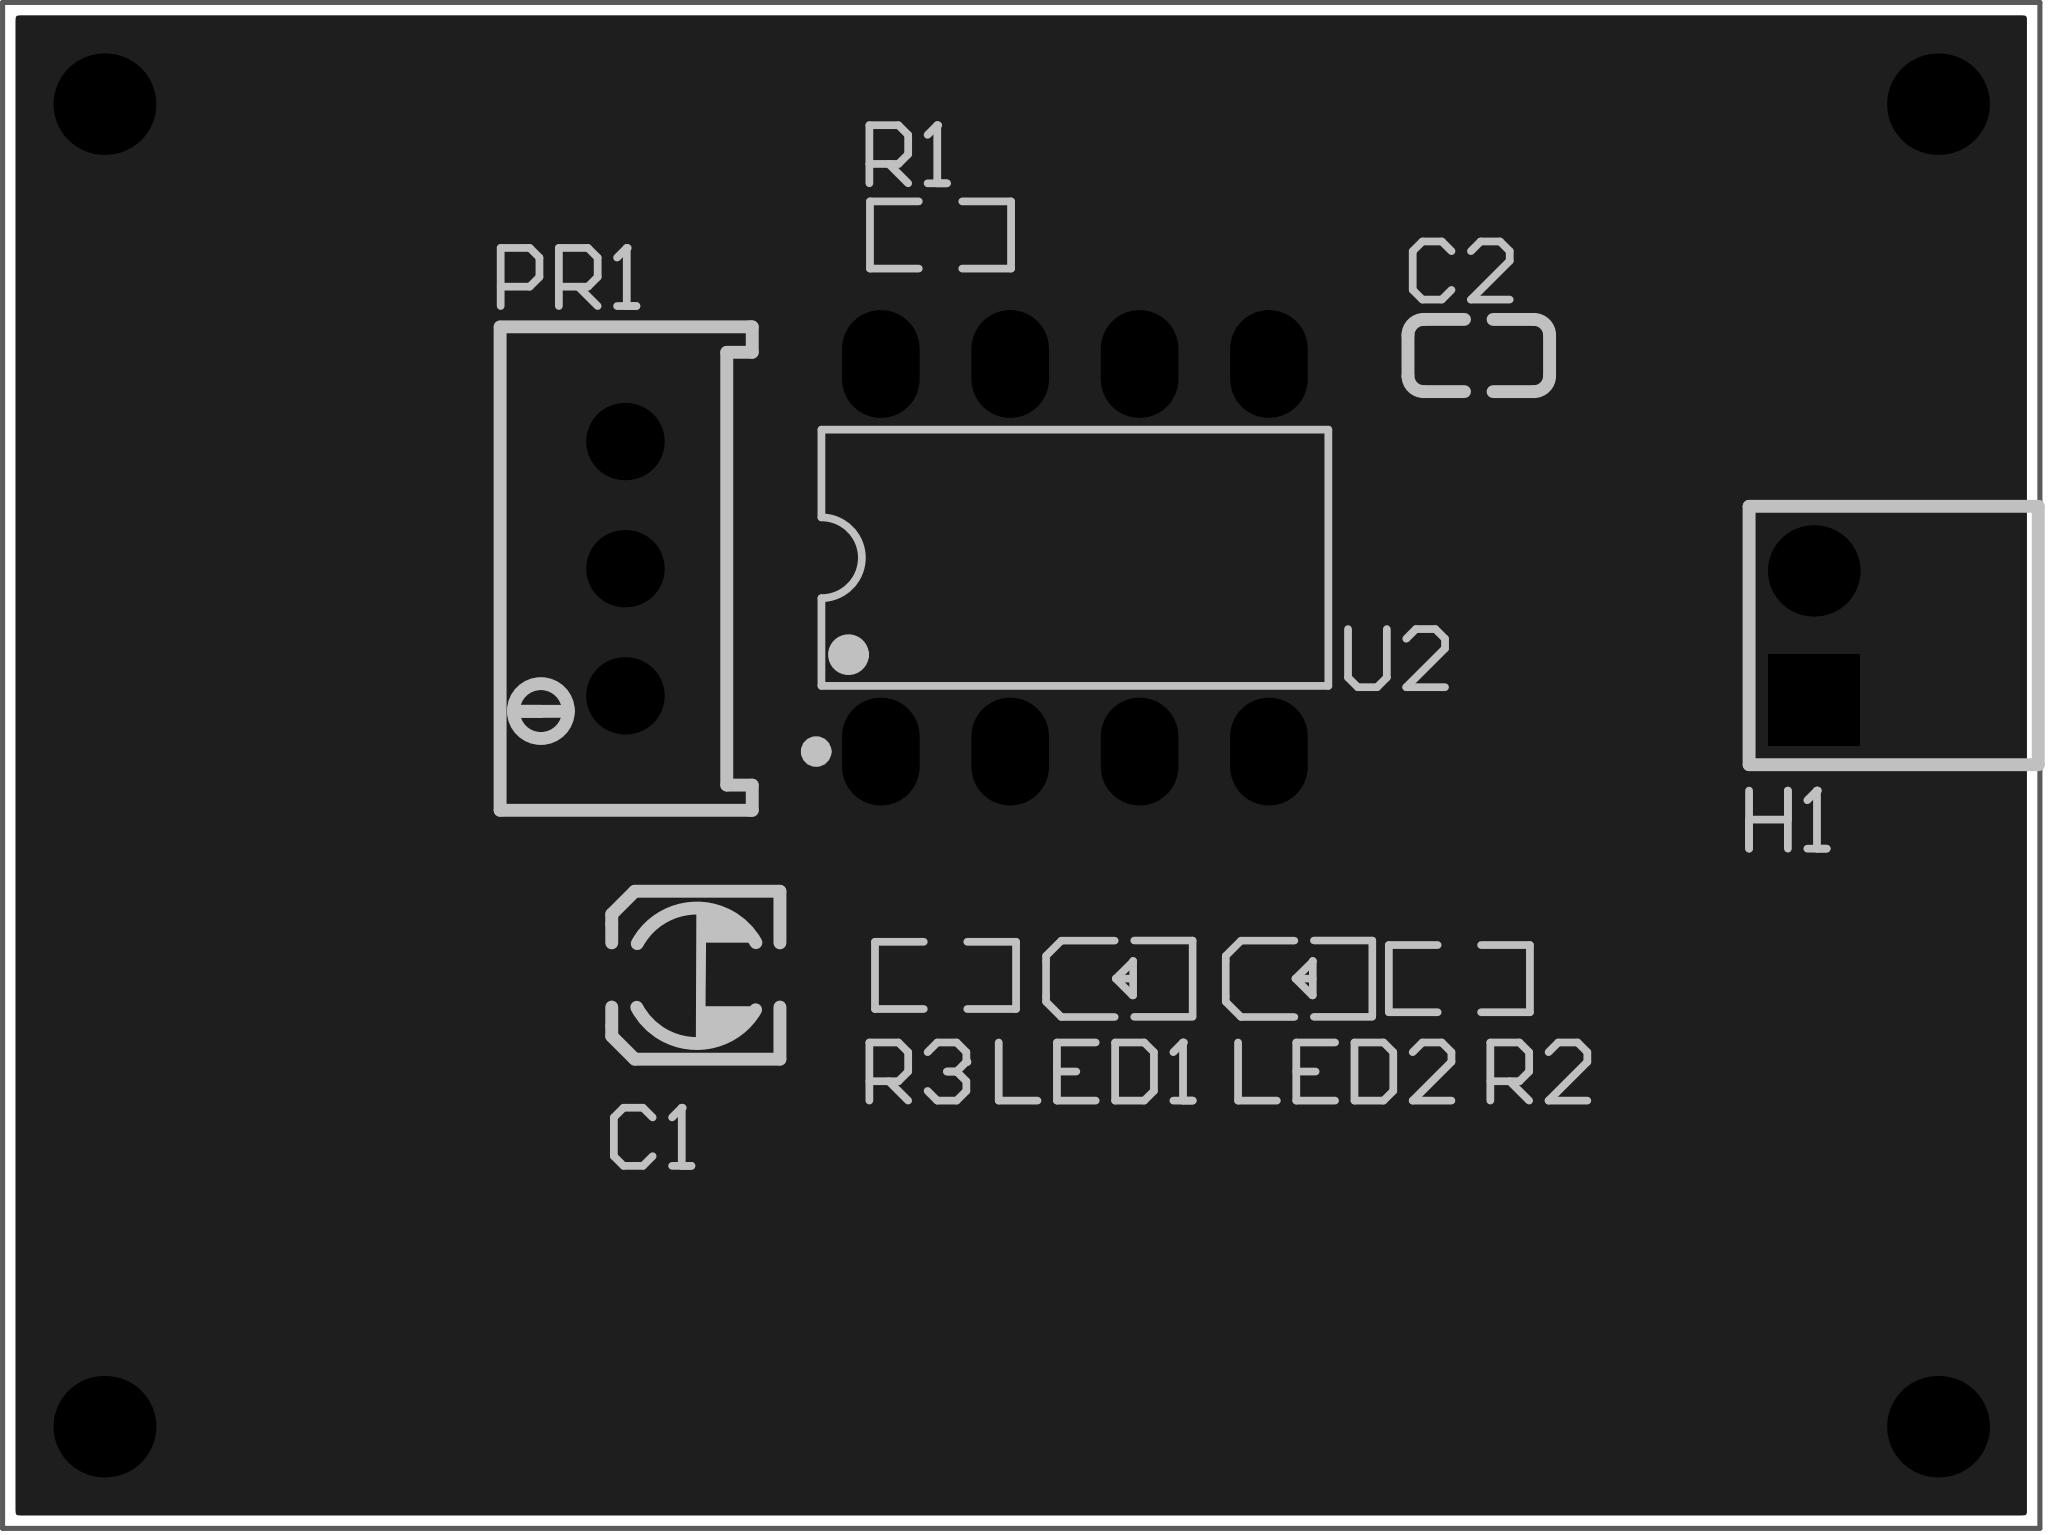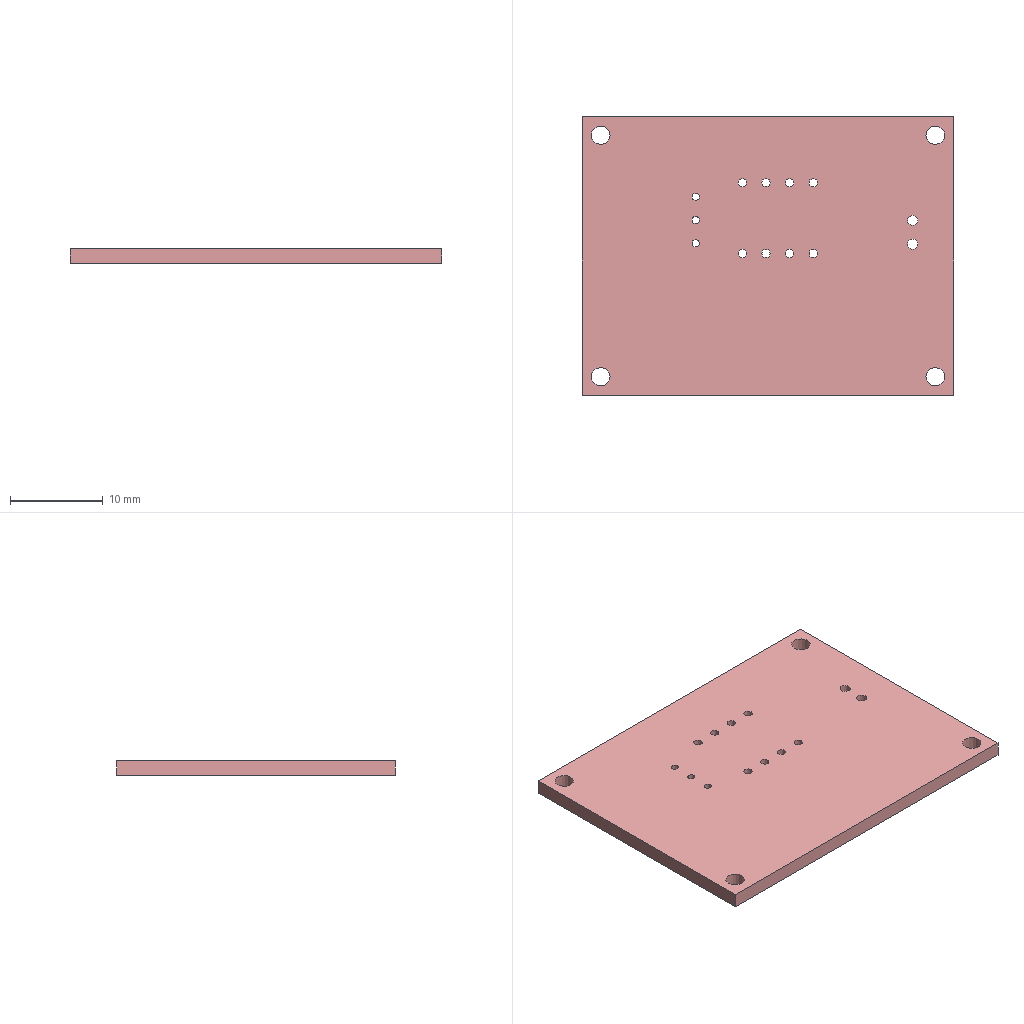Circuit board layout | Altium Designer | box 40 x 30 x 1.6 mm
Layer stack:
# Altium Designer layer stack of  (unit mm; dielectric type: 0 none, 1 core, 2 prepreg, 3 surface material)
index,name,kind,layer,copper_thickness_mm,dielectric_type,dielectric_thickness_mm,dielectric_material,dielectric_constant
0,Top Paste Mask Layer,other,,,,,,
1,Top Silkscreen Layer,other,,,,,,
2,Top Solder Mask Layer,dielectric,,,3,0.01,,3.3
3,Top Layer,copper,Top Layer,0.035,,,,
4,Dielectric1,dielectric,,,3,1.51,FR4,4.5
5,Bottom Layer,copper,Bottom Layer,0.035,,,,
6,Bottom Solder Mask Layer,dielectric,,,3,0.01,,3.3
7,Bottom Silkscreen Layer,other,,,,,,
8,Bottom Paste Mask Layer,other,,,,,,
# drill layer pairs: low layer,high layer
drill_pair,Top Layer,Bottom Layer
Part placement:
Designator,Comment,Layer,Footprint,Center-X(mm),Center-Y(mm),Rotation
R1,4.7K,TopLayer,R0603,94.615,101.628,180
R3,100,TopLayer,R0603,94.713,87.072,0
U2,NE555,TopLayer,DIP-8_L9.8-W6.4-P2.54-LS7.6-BL,97.253,95.282,0
LED1,,TopLayer,LED_0603,98.176,87.001,0
C1,10uF,TopLayer,C_Ele_SMD_3x5.4mm,89.811,87.08,180
C2,103,TopLayer,C0603,105.183,99.258,180
PR1,100kΩ,TopLayer,R_3296,88.419,95.067,90
LED2,,TopLayer,LED_0603,101.703,87.001,0
R2,1K,TopLayer,R0603,104.802,87.008,0
H1,,TopLayer,HDR-TH_2P-P2.54-V-M-1,111.76,93.754,90
Pad and via stacks:
# Altium Designer via and pad stacks of  (unit mm). Each distinct definition once, with the count of objects using it.
# via: kind,start_layer,end_layer,hole_mm,diameter_mm,mode(0 simple;1 top-mid-bottom;2 full stack),diameter_per_layer,count,example_net
# pad: kind,layer,hole_mm,hole_type(0 round;1 square;2 slot),plating,top_size,top_shape(1 round;2 rect;3 octagon;9 rounded rect),mid_size,bottom_size,mode,footprint,size_per_layer,count,example
pad,Multi-Layer,2,0,plated,2x2,1,2x2,2x2,0,,,4,1
pad,Multi-Layer,0.9,0,plated,1.524x2.125,1,1.524x2.125,1.524x2.125,0,DIP-8_L9.8-W6.4-P2.54-LS7.6-BL,,8,U2.1
pad,Multi-Layer,0.762,0,plated,1.524x1.524,1,1.524x1.524,1.524x1.524,0,R_3296,,3,PR1.2
pad,Multi-Layer,1.1,0,plated,1.8x1.8,1,1.8x1.8,1.8x1.8,0,HDR-TH_2P-P2.54-V-M-1,,1,H1.2
pad,Multi-Layer,1.1,0,plated,1.8x1.8,2,1.8x1.8,1.8x1.8,0,HDR-TH_2P-P2.54-V-M-1,,1,H1.1
pad,Top Layer,0,0,plated,0.8065x0.864,2,0.8065x0.864,0.8065x0.864,0,R0603,,6,R1.2
pad,Top Layer,0,0,plated,0.8001x0.8001,2,0.8001x0.8001,0.8001x0.8001,0,LED_0603,,4,LED1.1
pad,Top Layer,0,0,plated,1.999x0.8001,2,1.999x0.8001,1.999x0.8001,0,C_Ele_SMD_3x5.4mm,,2,C1.1
pad,Top Layer,0,0,plated,0.8x0.9,2,0.8x0.9,0.8x0.9,0,C0603,,2,C2.2
Copper pours:
name,layer,net,type(0 solid;1 hatched;2 none)
Top Layer-GND,Top Layer,GND,0
Bottom Layer-GND,Bottom Layer,GND,0
Design rules, without the lines most boards share:
# Altium Designer design rules of  (exported by Altium Designer, unit mm)
# columns: name | kind | enabled | priority | scope1 | scope2 | descriptor | typed fields (field=value)
creepage | 65 | enabled | 1 | All | All | Creepage Distance Constraint =(0mil) (All),(All) |